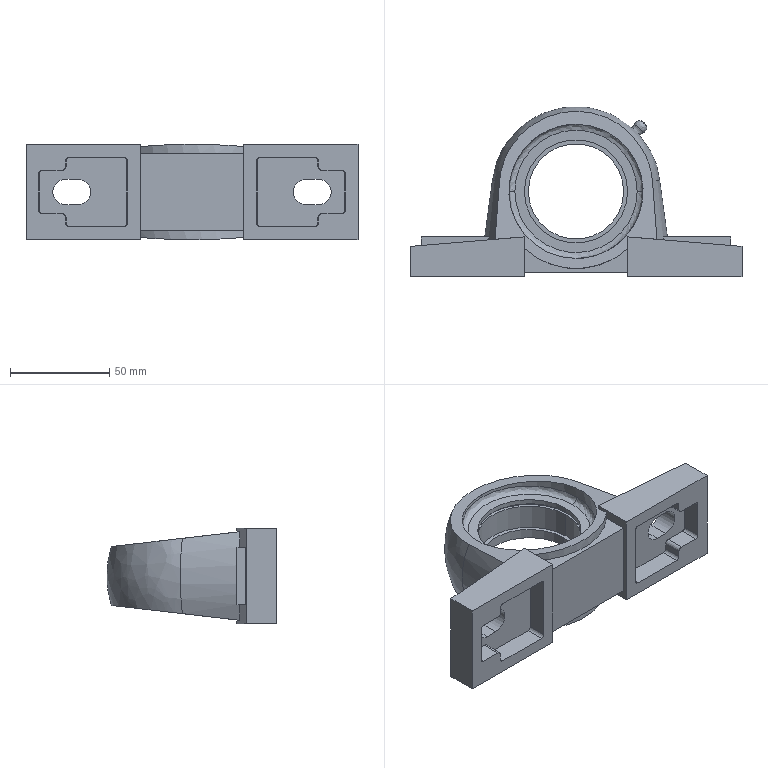Part | SolidWorks | features BaseBody 1 | 1 solid | 100 faces | box 167 x 85.5 x 48 mm | volume 186208 mm3 | plane 53 | cylinder 18 | cone 16 | spline 13 | commonest cylinder face diameters 13 x4 52 x4 67.524 x4 48 x2 55 x2 77.659 x2